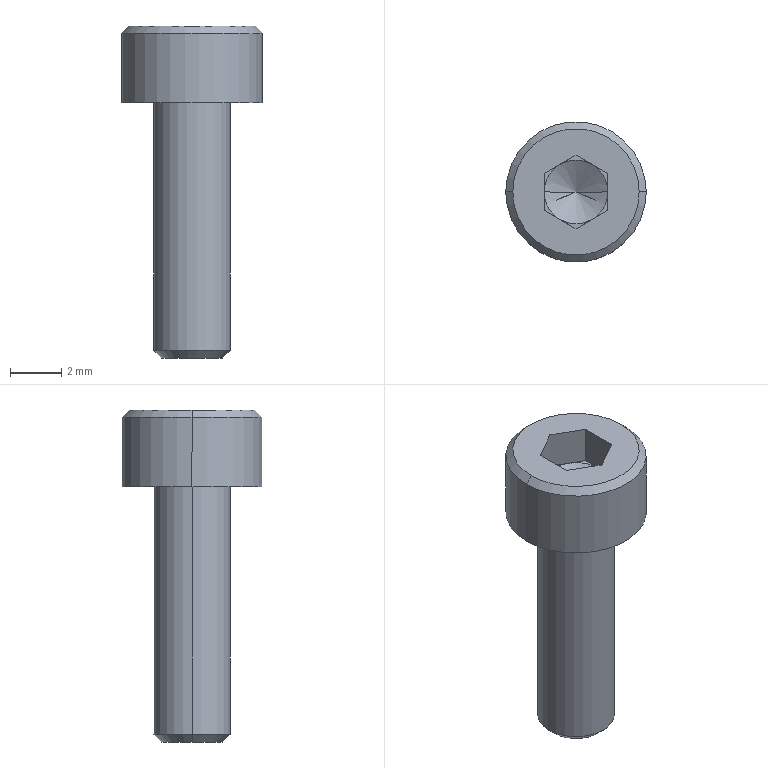Part | NX | features BREP 1 | 1 solid | 25 faces | box 5.5 x 5.5 x 13 mm | volume 131.617 mm3 | plane 15 | cone 6 | cylinder 4 | commonest cylinder face diameters 3 x2 5.5 x2
STEP:
#1=CARTESIAN_POINT('',(0.,0.,0.7783));
#2=VERTEX_POINT('',#1);
#3=CARTESIAN_POINT('',(1.25,0.,1.5));
#4=VERTEX_POINT('',#3);
#5=CARTESIAN_POINT('',(0.,0.,0.7783));
#6=DIRECTION('',(0.866,0.,0.5));
#7=VECTOR('',#6,1000.);
#8=LINE('',#5,#7);
#9=EDGE_CURVE('',#2,#4,#8,.T.);
#10=ORIENTED_EDGE('',*,*,#9,.F.);
#11=CARTESIAN_POINT('',(-1.25,0.,1.5));
#12=VERTEX_POINT('',#11);
#13=CARTESIAN_POINT('',(0.,0.,0.7783));
#14=DIRECTION('',(-0.866,0.,0.5));
#15=VECTOR('',#14,1000.);
#16=LINE('',#13,#15);
#17=EDGE_CURVE('',#2,#12,#16,.T.);
#18=ORIENTED_EDGE('',*,*,#17,.T.);
#19=CARTESIAN_POINT('',(-0.625,-1.083,1.5));
#20=VERTEX_POINT('',#19);
#21=CARTESIAN_POINT('',(0.,0.,1.5));
#22=DIRECTION('',(0.,0.,1.));
#23=DIRECTION('',(1.,0.,0.));
#24=AXIS2_PLACEMENT_3D('',#21,#22,#23);
#25=CIRCLE('',#24,1.25);
#26=EDGE_CURVE('',#12,#20,#25,.T.);
#27=ORIENTED_EDGE('',*,*,#26,.T.);
#28=CARTESIAN_POINT('',(0.625,-1.083,1.5));
#29=VERTEX_POINT('',#28);
#30=CARTESIAN_POINT('',(0.,0.,1.5));
#31=DIRECTION('',(0.,0.,1.));
#32=DIRECTION('',(1.,0.,0.));
#33=AXIS2_PLACEMENT_3D('',#30,#31,#32);
#34=CIRCLE('',#33,1.25);
#35=EDGE_CURVE('',#20,#29,#34,.T.);
#36=ORIENTED_EDGE('',*,*,#35,.T.);
#37=CARTESIAN_POINT('',(0.,0.,1.5));
#38=DIRECTION('',(0.,0.,1.));
#39=DIRECTION('',(1.,0.,0.));
#40=AXIS2_PLACEMENT_3D('',#37,#38,#39);
#41=CIRCLE('',#40,1.25);
#42=EDGE_CURVE('',#29,#4,#41,.T.);
#43=ORIENTED_EDGE('',*,*,#42,.T.);
#44=EDGE_LOOP('',(#10,#18,#27,#36,#43));
#45=FACE_BOUND('',#44,.T.);
#46=CARTESIAN_POINT('',(0.,0.,1000.778));
#47=DIRECTION('',(0.,0.,1.));
#48=DIRECTION('',(-1.,0.,0.));
#49=AXIS2_PLACEMENT_3D('',#46,#47,#48);
#50=CONICAL_SURFACE('',#49,1732.051,1.047);
#51=ADVANCED_FACE('',(#45),#50,.F.);
#52=CARTESIAN_POINT('',(2.75,0.,0.));
#53=VERTEX_POINT('',#52);
#54=CARTESIAN_POINT('',(-2.75,0.,0.));
#55=VERTEX_POINT('',#54);
#56=CARTESIAN_POINT('',(0.,0.,0.));
#57=DIRECTION('',(0.,0.,1.));
#58=DIRECTION('',(1.,0.,0.));
#59=AXIS2_PLACEMENT_3D('',#56,#57,#58);
#60=CIRCLE('',#59,2.75);
#61=EDGE_CURVE('',#53,#55,#60,.T.);
#62=ORIENTED_EDGE('',*,*,#61,.T.);
#63=CARTESIAN_POINT('',(-2.75,0.,2.725));
#64=VERTEX_POINT('',#63);
#65=CARTESIAN_POINT('',(-2.75,0.,0.));
#66=DIRECTION('',(0.,0.,1.));
#67=VECTOR('',#66,1000.);
#68=LINE('',#65,#67);
#69=EDGE_CURVE('',#55,#64,#68,.T.);
#70=ORIENTED_EDGE('',*,*,#69,.T.);
#71=CARTESIAN_POINT('',(2.75,0.,2.725));
#72=VERTEX_POINT('',#71);
#73=CARTESIAN_POINT('',(0.,0.,2.725));
#74=DIRECTION('',(0.,0.,1.));
#75=DIRECTION('',(1.,0.,0.));
#76=AXIS2_PLACEMENT_3D('',#73,#74,#75);
#77=CIRCLE('',#76,2.75);
#78=EDGE_CURVE('',#72,#64,#77,.T.);
#79=ORIENTED_EDGE('',*,*,#78,.F.);
#80=CARTESIAN_POINT('',(2.75,0.,0.));
#81=DIRECTION('',(0.,0.,1.));
#82=VECTOR('',#81,1000.);
#83=LINE('',#80,#82);
#84=EDGE_CURVE('',#53,#72,#83,.T.);
#85=ORIENTED_EDGE('',*,*,#84,.F.);
#86=EDGE_LOOP('',(#62,#70,#79,#85));
#87=FACE_BOUND('',#86,.T.);
#88=CARTESIAN_POINT('',(0.,0.,0.));
#89=DIRECTION('',(0.,0.,1.));
#90=DIRECTION('',(-1.,0.,0.));
#91=AXIS2_PLACEMENT_3D('',#88,#89,#90);
#92=CYLINDRICAL_SURFACE('',#91,2.75);
#93=ADVANCED_FACE('',(#87),#92,.T.);
#94=CARTESIAN_POINT('',(2.475,0.,3.));
#95=VERTEX_POINT('',#94);
#96=CARTESIAN_POINT('',(-2.475,0.,3.));
#97=VERTEX_POINT('',#96);
#98=CARTESIAN_POINT('',(0.,0.,3.));
#99=DIRECTION('',(0.,0.,1.));
#100=DIRECTION('',(1.,0.,0.));
#101=AXIS2_PLACEMENT_3D('',#98,#99,#100);
#102=CIRCLE('',#101,2.475);
#103=EDGE_CURVE('',#95,#97,#102,.T.);
#104=ORIENTED_EDGE('',*,*,#103,.F.);
#105=CARTESIAN_POINT('',(2.75,0.,2.725));
#106=DIRECTION('',(0.7071,0.,-0.7071));
#107=VECTOR('',#106,1000.);
#108=LINE('',#105,#107);
#109=EDGE_CURVE('',#72,#95,#108,.F.);
#110=ORIENTED_EDGE('',*,*,#109,.F.);
#111=ORIENTED_EDGE('',*,*,#78,.T.);
#112=CARTESIAN_POINT('',(-2.75,0.,2.725));
#113=DIRECTION('',(-0.7071,0.,-0.7071));
#114=VECTOR('',#113,1000.);
#115=LINE('',#112,#114);
#116=EDGE_CURVE('',#64,#97,#115,.F.);
#117=ORIENTED_EDGE('',*,*,#116,.T.);
#118=EDGE_LOOP('',(#104,#110,#111,#117));
#119=FACE_BOUND('',#118,.T.);
#120=CARTESIAN_POINT('',(0.,0.,2.725));
#121=DIRECTION('',(0.,0.,-1.));
#122=DIRECTION('',(1.,0.,0.));
#123=AXIS2_PLACEMENT_3D('',#120,#121,#122);
#124=CONICAL_SURFACE('',#123,2.75,0.7854);
#125=ADVANCED_FACE('',(#119),#124,.T.);
#126=CARTESIAN_POINT('',(1.194,0.,-10.));
#127=VERTEX_POINT('',#126);
#128=CARTESIAN_POINT('',(-1.194,0.,-10.));
#129=VERTEX_POINT('',#128);
#130=CARTESIAN_POINT('',(0.,0.,-10.));
#131=DIRECTION('',(0.,0.,1.));
#132=DIRECTION('',(1.,0.,0.));
#133=AXIS2_PLACEMENT_3D('',#130,#131,#132);
#134=CIRCLE('',#133,1.194);
#135=EDGE_CURVE('',#127,#129,#134,.T.);
#136=ORIENTED_EDGE('',*,*,#135,.T.);
#137=CARTESIAN_POINT('',(-1.5,0.,-9.694));
#138=VERTEX_POINT('',#137);
#139=CARTESIAN_POINT('',(-1.194,0.,-10.));
#140=DIRECTION('',(-0.7071,0.,0.7071));
#141=VECTOR('',#140,1000.);
#142=LINE('',#139,#141);
#143=EDGE_CURVE('',#129,#138,#142,.T.);
#144=ORIENTED_EDGE('',*,*,#143,.T.);
#145=CARTESIAN_POINT('',(1.5,0.,-9.694));
#146=VERTEX_POINT('',#145);
#147=CARTESIAN_POINT('',(0.,0.,-9.694));
#148=DIRECTION('',(0.,0.,1.));
#149=DIRECTION('',(1.,0.,0.));
#150=AXIS2_PLACEMENT_3D('',#147,#148,#149);
#151=CIRCLE('',#150,1.5);
#152=EDGE_CURVE('',#146,#138,#151,.T.);
#153=ORIENTED_EDGE('',*,*,#152,.F.);
#154=CARTESIAN_POINT('',(1.194,0.,-10.));
#155=DIRECTION('',(0.7071,0.,0.7071));
#156=VECTOR('',#155,1000.);
#157=LINE('',#154,#156);
#158=EDGE_CURVE('',#127,#146,#157,.T.);
#159=ORIENTED_EDGE('',*,*,#158,.F.);
#160=EDGE_LOOP('',(#136,#144,#153,#159));
#161=FACE_BOUND('',#160,.T.);
#162=CARTESIAN_POINT('',(0.,0.,-10.));
#163=DIRECTION('',(0.,0.,1.));
#164=DIRECTION('',(-1.,0.,0.));
#165=AXIS2_PLACEMENT_3D('',#162,#163,#164);
#166=CONICAL_SURFACE('',#165,1.194,0.7854);
#167=ADVANCED_FACE('',(#161),#166,.T.);
#168=ORIENTED_EDGE('',*,*,#152,.T.);
#169=CARTESIAN_POINT('',(-1.5,0.,0.));
#170=VERTEX_POINT('',#169);
#171=CARTESIAN_POINT('',(-1.5,0.,-10.));
#172=DIRECTION('',(0.,0.,1.));
#173=VECTOR('',#172,1000.);
#174=LINE('',#171,#173);
#175=EDGE_CURVE('',#138,#170,#174,.T.);
#176=ORIENTED_EDGE('',*,*,#175,.T.);
#177=CARTESIAN_POINT('',(1.5,0.,0.));
#178=VERTEX_POINT('',#177);
#179=CARTESIAN_POINT('',(0.,0.,0.));
#180=DIRECTION('',(0.,0.,1.));
#181=DIRECTION('',(1.,0.,0.));
#182=AXIS2_PLACEMENT_3D('',#179,#180,#181);
#183=CIRCLE('',#182,1.5);
#184=EDGE_CURVE('',#178,#170,#183,.T.);
#185=ORIENTED_EDGE('',*,*,#184,.F.);
#186=CARTESIAN_POINT('',(1.5,0.,-10.));
#187=DIRECTION('',(0.,0.,1.));
#188=VECTOR('',#187,1000.);
#189=LINE('',#186,#188);
#190=EDGE_CURVE('',#146,#178,#189,.T.);
#191=ORIENTED_EDGE('',*,*,#190,.F.);
#192=EDGE_LOOP('',(#168,#176,#185,#191));
#193=FACE_BOUND('',#192,.T.);
#194=CARTESIAN_POINT('',(0.,0.,-10.));
#195=DIRECTION('',(0.,0.,1.));
#196=DIRECTION('',(-1.,0.,0.));
#197=AXIS2_PLACEMENT_3D('',#194,#195,#196);
#198=CYLINDRICAL_SURFACE('',#197,1.5);
#199=ADVANCED_FACE('',(#193),#198,.T.);
#200=CARTESIAN_POINT('',(0.625,1.083,1.5));
#201=VERTEX_POINT('',#200);
#202=CARTESIAN_POINT('',(0.,0.,1.5));
#203=DIRECTION('',(0.,0.,1.));
#204=DIRECTION('',(1.,0.,0.));
#205=AXIS2_PLACEMENT_3D('',#202,#203,#204);
#206=CIRCLE('',#205,1.25);
#207=EDGE_CURVE('',#4,#201,#206,.T.);
#208=ORIENTED_EDGE('',*,*,#207,.F.);
#209=CARTESIAN_POINT('',(1.25,0.7217,1.5));
#210=VERTEX_POINT('',#209);
#211=CARTESIAN_POINT('',(1.25,-0.7217,1.5));
#212=DIRECTION('',(0.,1.,0.));
#213=VECTOR('',#212,1000.);
#214=LINE('',#211,#213);
#215=EDGE_CURVE('',#4,#210,#214,.T.);
#216=ORIENTED_EDGE('',*,*,#215,.T.);
#217=CARTESIAN_POINT('',(1.25,0.7217,1.5));
#218=DIRECTION('',(-0.866,0.5,0.));
#219=VECTOR('',#218,1000.);
#220=LINE('',#217,#219);
#221=EDGE_CURVE('',#210,#201,#220,.T.);
#222=ORIENTED_EDGE('',*,*,#221,.T.);
#223=EDGE_LOOP('',(#208,#216,#222));
#224=FACE_BOUND('',#223,.T.);
#225=CARTESIAN_POINT('',(0.,0.,1.5));
#226=DIRECTION('',(0.,0.,1.));
#227=DIRECTION('',(-1.,0.,0.));
#228=AXIS2_PLACEMENT_3D('',#225,#226,#227);
#229=PLANE('',#228);
#230=ADVANCED_FACE('',(#224),#229,.T.);
#231=CARTESIAN_POINT('',(-0.625,1.083,1.5));
#232=VERTEX_POINT('',#231);
#233=CARTESIAN_POINT('',(0.,0.,1.5));
#234=DIRECTION('',(0.,0.,1.));
#235=DIRECTION('',(1.,0.,0.));
#236=AXIS2_PLACEMENT_3D('',#233,#234,#235);
#237=CIRCLE('',#236,1.25);
#238=EDGE_CURVE('',#201,#232,#237,.T.);
#239=ORIENTED_EDGE('',*,*,#238,.F.);
#240=CARTESIAN_POINT('',(0.,1.443,1.5));
#241=VERTEX_POINT('',#240);
#242=CARTESIAN_POINT('',(1.25,0.7217,1.5));
#243=DIRECTION('',(-0.866,0.5,0.));
#244=VECTOR('',#243,1000.);
#245=LINE('',#242,#244);
#246=EDGE_CURVE('',#201,#241,#245,.T.);
#247=ORIENTED_EDGE('',*,*,#246,.T.);
#248=CARTESIAN_POINT('',(0.,1.443,1.5));
#249=DIRECTION('',(-0.866,-0.5,0.));
#250=VECTOR('',#249,1000.);
#251=LINE('',#248,#250);
#252=EDGE_CURVE('',#241,#232,#251,.T.);
#253=ORIENTED_EDGE('',*,*,#252,.T.);
#254=EDGE_LOOP('',(#239,#247,#253));
#255=FACE_BOUND('',#254,.T.);
#256=CARTESIAN_POINT('',(0.,0.,1.5));
#257=DIRECTION('',(0.,0.,1.));
#258=DIRECTION('',(-1.,0.,0.));
#259=AXIS2_PLACEMENT_3D('',#256,#257,#258);
#260=PLANE('',#259);
#261=ADVANCED_FACE('',(#255),#260,.T.);
#262=CARTESIAN_POINT('',(0.,0.,1.5));
#263=DIRECTION('',(0.,0.,1.));
#264=DIRECTION('',(1.,0.,0.));
#265=AXIS2_PLACEMENT_3D('',#262,#263,#264);
#266=CIRCLE('',#265,1.25);
#267=EDGE_CURVE('',#232,#12,#266,.T.);
#268=ORIENTED_EDGE('',*,*,#267,.F.);
#269=CARTESIAN_POINT('',(-1.25,0.7217,1.5));
#270=VERTEX_POINT('',#269);
#271=CARTESIAN_POINT('',(0.,1.443,1.5));
#272=DIRECTION('',(-0.866,-0.5,0.));
#273=VECTOR('',#272,1000.);
#274=LINE('',#271,#273);
#275=EDGE_CURVE('',#232,#270,#274,.T.);
#276=ORIENTED_EDGE('',*,*,#275,.T.);
#277=CARTESIAN_POINT('',(-1.25,0.7217,1.5));
#278=DIRECTION('',(0.,-1.,0.));
#279=VECTOR('',#278,1000.);
#280=LINE('',#277,#279);
#281=EDGE_CURVE('',#270,#12,#280,.T.);
#282=ORIENTED_EDGE('',*,*,#281,.T.);
#283=EDGE_LOOP('',(#268,#276,#282));
#284=FACE_BOUND('',#283,.T.);
#285=CARTESIAN_POINT('',(0.,0.,1.5));
#286=DIRECTION('',(0.,0.,1.));
#287=DIRECTION('',(-1.,0.,0.));
#288=AXIS2_PLACEMENT_3D('',#285,#286,#287);
#289=PLANE('',#288);
#290=ADVANCED_FACE('',(#284),#289,.T.);
#291=ORIENTED_EDGE('',*,*,#26,.F.);
#292=CARTESIAN_POINT('',(-1.25,-0.7217,1.5));
#293=VERTEX_POINT('',#292);
#294=CARTESIAN_POINT('',(-1.25,0.7217,1.5));
#295=DIRECTION('',(0.,-1.,0.));
#296=VECTOR('',#295,1000.);
#297=LINE('',#294,#296);
#298=EDGE_CURVE('',#12,#293,#297,.T.);
#299=ORIENTED_EDGE('',*,*,#298,.T.);
#300=CARTESIAN_POINT('',(-1.25,-0.7217,1.5));
#301=DIRECTION('',(0.866,-0.5,0.));
#302=VECTOR('',#301,1000.);
#303=LINE('',#300,#302);
#304=EDGE_CURVE('',#293,#20,#303,.T.);
#305=ORIENTED_EDGE('',*,*,#304,.T.);
#306=EDGE_LOOP('',(#291,#299,#305));
#307=FACE_BOUND('',#306,.T.);
#308=CARTESIAN_POINT('',(0.,0.,1.5));
#309=DIRECTION('',(0.,0.,1.));
#310=DIRECTION('',(-1.,0.,0.));
#311=AXIS2_PLACEMENT_3D('',#308,#309,#310);
#312=PLANE('',#311);
#313=ADVANCED_FACE('',(#307),#312,.T.);
#314=ORIENTED_EDGE('',*,*,#35,.F.);
#315=CARTESIAN_POINT('',(0.,-1.443,1.5));
#316=VERTEX_POINT('',#315);
#317=CARTESIAN_POINT('',(-1.25,-0.7217,1.5));
#318=DIRECTION('',(0.866,-0.5,0.));
#319=VECTOR('',#318,1000.);
#320=LINE('',#317,#319);
#321=EDGE_CURVE('',#20,#316,#320,.T.);
#322=ORIENTED_EDGE('',*,*,#321,.T.);
#323=CARTESIAN_POINT('',(0.,-1.443,1.5));
#324=DIRECTION('',(0.866,0.5,0.));
#325=VECTOR('',#324,1000.);
#326=LINE('',#323,#325);
#327=EDGE_CURVE('',#316,#29,#326,.T.);
#328=ORIENTED_EDGE('',*,*,#327,.T.);
#329=EDGE_LOOP('',(#314,#322,#328));
#330=FACE_BOUND('',#329,.T.);
#331=CARTESIAN_POINT('',(0.,0.,1.5));
#332=DIRECTION('',(0.,0.,1.));
#333=DIRECTION('',(-1.,0.,0.));
#334=AXIS2_PLACEMENT_3D('',#331,#332,#333);
#335=PLANE('',#334);
#336=ADVANCED_FACE('',(#330),#335,.T.);
#337=ORIENTED_EDGE('',*,*,#175,.F.);
#338=CARTESIAN_POINT('',(0.,0.,-9.694));
#339=DIRECTION('',(0.,0.,1.));
#340=DIRECTION('',(1.,0.,0.));
#341=AXIS2_PLACEMENT_3D('',#338,#339,#340);
#342=CIRCLE('',#341,1.5);
#343=EDGE_CURVE('',#138,#146,#342,.T.);
#344=ORIENTED_EDGE('',*,*,#343,.T.);
#345=ORIENTED_EDGE('',*,*,#190,.T.);
#346=CARTESIAN_POINT('',(0.,0.,0.));
#347=DIRECTION('',(0.,0.,1.));
#348=DIRECTION('',(1.,0.,0.));
#349=AXIS2_PLACEMENT_3D('',#346,#347,#348);
#350=CIRCLE('',#349,1.5);
#351=EDGE_CURVE('',#170,#178,#350,.T.);
#352=ORIENTED_EDGE('',*,*,#351,.F.);
#353=EDGE_LOOP('',(#337,#344,#345,#352));
#354=FACE_BOUND('',#353,.T.);
#355=CARTESIAN_POINT('',(0.,0.,-10.));
#356=DIRECTION('',(0.,0.,1.));
#357=DIRECTION('',(-1.,0.,0.));
#358=AXIS2_PLACEMENT_3D('',#355,#356,#357);
#359=CYLINDRICAL_SURFACE('',#358,1.5);
#360=ADVANCED_FACE('',(#354),#359,.T.);
#361=ORIENTED_EDGE('',*,*,#143,.F.);
#362=CARTESIAN_POINT('',(0.,0.,-10.));
#363=DIRECTION('',(0.,0.,1.));
#364=DIRECTION('',(1.,0.,0.));
#365=AXIS2_PLACEMENT_3D('',#362,#363,#364);
#366=CIRCLE('',#365,1.194);
#367=EDGE_CURVE('',#129,#127,#366,.T.);
#368=ORIENTED_EDGE('',*,*,#367,.T.);
#369=ORIENTED_EDGE('',*,*,#158,.T.);
#370=ORIENTED_EDGE('',*,*,#343,.F.);
#371=EDGE_LOOP('',(#361,#368,#369,#370));
#372=FACE_BOUND('',#371,.T.);
#373=CARTESIAN_POINT('',(0.,0.,-10.));
#374=DIRECTION('',(0.,0.,1.));
#375=DIRECTION('',(-1.,0.,0.));
#376=AXIS2_PLACEMENT_3D('',#373,#374,#375);
#377=CONICAL_SURFACE('',#376,1.194,0.7854);
#378=ADVANCED_FACE('',(#372),#377,.T.);
#379=ORIENTED_EDGE('',*,*,#135,.F.);
#380=ORIENTED_EDGE('',*,*,#367,.F.);
#381=EDGE_LOOP('',(#379,#380));
#382=FACE_BOUND('',#381,.T.);
#383=CARTESIAN_POINT('',(0.,1.194,-10.));
#384=DIRECTION('',(0.,0.,1.));
#385=DIRECTION('',(-1.,0.,0.));
#386=AXIS2_PLACEMENT_3D('',#383,#384,#385);
#387=PLANE('',#386);
#388=ADVANCED_FACE('',(#382),#387,.F.);
#389=CARTESIAN_POINT('',(0.,-1.443,3.));
#390=VERTEX_POINT('',#389);
#391=CARTESIAN_POINT('',(1.25,-0.7217,3.));
#392=VERTEX_POINT('',#391);
#393=CARTESIAN_POINT('',(0.,-1.443,3.));
#394=DIRECTION('',(0.866,0.5,0.));
#395=VECTOR('',#394,1000.);
#396=LINE('',#393,#395);
#397=EDGE_CURVE('',#390,#392,#396,.T.);
#398=ORIENTED_EDGE('',*,*,#397,.F.);
#399=CARTESIAN_POINT('',(-1.25,-0.7217,3.));
#400=VERTEX_POINT('',#399);
#401=CARTESIAN_POINT('',(-1.25,-0.7217,3.));
#402=DIRECTION('',(0.866,-0.5,0.));
#403=VECTOR('',#402,1000.);
#404=LINE('',#401,#403);
#405=EDGE_CURVE('',#400,#390,#404,.T.);
#406=ORIENTED_EDGE('',*,*,#405,.F.);
#407=CARTESIAN_POINT('',(-1.25,0.7217,3.));
#408=VERTEX_POINT('',#407);
#409=CARTESIAN_POINT('',(-1.25,0.7217,3.));
#410=DIRECTION('',(0.,-1.,0.));
#411=VECTOR('',#410,1000.);
#412=LINE('',#409,#411);
#413=EDGE_CURVE('',#408,#400,#412,.T.);
#414=ORIENTED_EDGE('',*,*,#413,.F.);
#415=CARTESIAN_POINT('',(0.,1.443,3.));
#416=VERTEX_POINT('',#415);
#417=CARTESIAN_POINT('',(0.,1.443,3.));
#418=DIRECTION('',(-0.866,-0.5,0.));
#419=VECTOR('',#418,1000.);
#420=LINE('',#417,#419);
#421=EDGE_CURVE('',#416,#408,#420,.T.);
#422=ORIENTED_EDGE('',*,*,#421,.F.);
#423=CARTESIAN_POINT('',(1.25,0.7217,3.));
#424=VERTEX_POINT('',#423);
#425=CARTESIAN_POINT('',(1.25,0.7217,3.));
#426=DIRECTION('',(-0.866,0.5,0.));
#427=VECTOR('',#426,1000.);
#428=LINE('',#425,#427);
#429=EDGE_CURVE('',#424,#416,#428,.T.);
#430=ORIENTED_EDGE('',*,*,#429,.F.);
#431=CARTESIAN_POINT('',(1.25,-0.7217,3.));
#432=DIRECTION('',(0.,1.,0.));
#433=VECTOR('',#432,1000.);
#434=LINE('',#431,#433);
#435=EDGE_CURVE('',#392,#424,#434,.T.);
#436=ORIENTED_EDGE('',*,*,#435,.F.);
#437=EDGE_LOOP('',(#398,#406,#414,#422,#430,#436));
#438=FACE_BOUND('',#437,.T.);
#439=CARTESIAN_POINT('',(0.,0.,3.));
#440=DIRECTION('',(0.,0.,1.));
#441=DIRECTION('',(1.,0.,0.));
#442=AXIS2_PLACEMENT_3D('',#439,#440,#441);
#443=CIRCLE('',#442,2.475);
#444=EDGE_CURVE('',#97,#95,#443,.T.);
#445=ORIENTED_EDGE('',*,*,#444,.T.);
#446=ORIENTED_EDGE('',*,*,#103,.T.);
#447=EDGE_LOOP('',(#445,#446));
#448=FACE_BOUND('',#447,.T.);
#449=CARTESIAN_POINT('',(0.,0.,3.));
#450=DIRECTION('',(0.,0.,-1.));
#451=DIRECTION('',(1.,0.,0.));
#452=AXIS2_PLACEMENT_3D('',#449,#450,#451);
#453=PLANE('',#452);
#454=ADVANCED_FACE('',(#438,#448),#453,.F.);
#455=ORIENTED_EDGE('',*,*,#109,.T.);
#456=ORIENTED_EDGE('',*,*,#444,.F.);
#457=ORIENTED_EDGE('',*,*,#116,.F.);
#458=CARTESIAN_POINT('',(0.,0.,2.725));
#459=DIRECTION('',(0.,0.,1.));
#460=DIRECTION('',(1.,0.,0.));
#461=AXIS2_PLACEMENT_3D('',#458,#459,#460);
#462=CIRCLE('',#461,2.75);
#463=EDGE_CURVE('',#64,#72,#462,.T.);
#464=ORIENTED_EDGE('',*,*,#463,.T.);
#465=EDGE_LOOP('',(#455,#456,#457,#464));
#466=FACE_BOUND('',#465,.T.);
#467=CARTESIAN_POINT('',(0.,0.,2.725));
#468=DIRECTION('',(0.,0.,-1.));
#469=DIRECTION('',(1.,0.,0.));
#470=AXIS2_PLACEMENT_3D('',#467,#468,#469);
#471=CONICAL_SURFACE('',#470,2.75,0.7854);
#472=ADVANCED_FACE('',(#466),#471,.T.);
#473=ORIENTED_EDGE('',*,*,#69,.F.);
#474=CARTESIAN_POINT('',(0.,0.,0.));
#475=DIRECTION('',(0.,0.,1.));
#476=DIRECTION('',(1.,0.,0.));
#477=AXIS2_PLACEMENT_3D('',#474,#475,#476);
#478=CIRCLE('',#477,2.75);
#479=EDGE_CURVE('',#55,#53,#478,.T.);
#480=ORIENTED_EDGE('',*,*,#479,.T.);
#481=ORIENTED_EDGE('',*,*,#84,.T.);
#482=ORIENTED_EDGE('',*,*,#463,.F.);
#483=EDGE_LOOP('',(#473,#480,#481,#482));
#484=FACE_BOUND('',#483,.T.);
#485=CARTESIAN_POINT('',(0.,0.,0.));
#486=DIRECTION('',(0.,0.,1.));
#487=DIRECTION('',(-1.,0.,0.));
#488=AXIS2_PLACEMENT_3D('',#485,#486,#487);
#489=CYLINDRICAL_SURFACE('',#488,2.75);
#490=ADVANCED_FACE('',(#484),#489,.T.);
#491=ORIENTED_EDGE('',*,*,#184,.T.);
#492=ORIENTED_EDGE('',*,*,#351,.T.);
#493=EDGE_LOOP('',(#491,#492));
#494=FACE_BOUND('',#493,.T.);
#495=ORIENTED_EDGE('',*,*,#61,.F.);
#496=ORIENTED_EDGE('',*,*,#479,.F.);
#497=EDGE_LOOP('',(#495,#496));
#498=FACE_BOUND('',#497,.T.);
#499=CARTESIAN_POINT('',(0.,2.75,0.));
#500=DIRECTION('',(0.,0.,1.));
#501=DIRECTION('',(-1.,0.,0.));
#502=AXIS2_PLACEMENT_3D('',#499,#500,#501);
#503=PLANE('',#502);
#504=ADVANCED_FACE('',(#494,#498),#503,.F.);
#505=ORIENTED_EDGE('',*,*,#405,.T.);
#506=CARTESIAN_POINT('',(0.,-1.443,1.5));
#507=DIRECTION('',(0.,0.,1.));
#508=VECTOR('',#507,1000.);
#509=LINE('',#506,#508);
#510=EDGE_CURVE('',#316,#390,#509,.T.);
#511=ORIENTED_EDGE('',*,*,#510,.F.);
#512=ORIENTED_EDGE('',*,*,#321,.F.);
#513=ORIENTED_EDGE('',*,*,#304,.F.);
#514=CARTESIAN_POINT('',(-1.25,-0.7217,1.5));
#515=DIRECTION('',(0.,0.,1.));
#516=VECTOR('',#515,1000.);
#517=LINE('',#514,#516);
#518=EDGE_CURVE('',#293,#400,#517,.T.);
#519=ORIENTED_EDGE('',*,*,#518,.T.);
#520=EDGE_LOOP('',(#505,#511,#512,#513,#519));
#521=FACE_BOUND('',#520,.T.);
#522=CARTESIAN_POINT('',(-1.25,-0.7217,1.5));
#523=DIRECTION('',(-0.5,-0.866,0.));
#524=DIRECTION('',(-0.866,0.5,0.));
#525=AXIS2_PLACEMENT_3D('',#522,#523,#524);
#526=PLANE('',#525);
#527=ADVANCED_FACE('',(#521),#526,.F.);
#528=ORIENTED_EDGE('',*,*,#413,.T.);
#529=ORIENTED_EDGE('',*,*,#518,.F.);
#530=ORIENTED_EDGE('',*,*,#298,.F.);
#531=ORIENTED_EDGE('',*,*,#281,.F.);
#532=CARTESIAN_POINT('',(-1.25,0.7217,1.5));
#533=DIRECTION('',(0.,0.,1.));
#534=VECTOR('',#533,1000.);
#535=LINE('',#532,#534);
#536=EDGE_CURVE('',#270,#408,#535,.T.);
#537=ORIENTED_EDGE('',*,*,#536,.T.);
#538=EDGE_LOOP('',(#528,#529,#530,#531,#537));
#539=FACE_BOUND('',#538,.T.);
#540=CARTESIAN_POINT('',(-1.25,0.7217,1.5));
#541=DIRECTION('',(-1.,0.,0.));
#542=DIRECTION('',(0.,0.,-1.));
#543=AXIS2_PLACEMENT_3D('',#540,#541,#542);
#544=PLANE('',#543);
#545=ADVANCED_FACE('',(#539),#544,.F.);
#546=ORIENTED_EDGE('',*,*,#421,.T.);
#547=ORIENTED_EDGE('',*,*,#536,.F.);
#548=ORIENTED_EDGE('',*,*,#275,.F.);
#549=ORIENTED_EDGE('',*,*,#252,.F.);
#550=CARTESIAN_POINT('',(0.,1.443,1.5));
#551=DIRECTION('',(0.,0.,1.));
#552=VECTOR('',#551,1000.);
#553=LINE('',#550,#552);
#554=EDGE_CURVE('',#241,#416,#553,.T.);
#555=ORIENTED_EDGE('',*,*,#554,.T.);
#556=EDGE_LOOP('',(#546,#547,#548,#549,#555));
#557=FACE_BOUND('',#556,.T.);
#558=CARTESIAN_POINT('',(0.,1.443,1.5));
#559=DIRECTION('',(-0.5,0.866,0.));
#560=DIRECTION('',(0.866,0.5,0.));
#561=AXIS2_PLACEMENT_3D('',#558,#559,#560);
#562=PLANE('',#561);
#563=ADVANCED_FACE('',(#557),#562,.F.);
#564=ORIENTED_EDGE('',*,*,#429,.T.);
#565=ORIENTED_EDGE('',*,*,#554,.F.);
#566=ORIENTED_EDGE('',*,*,#246,.F.);
#567=ORIENTED_EDGE('',*,*,#221,.F.);
#568=CARTESIAN_POINT('',(1.25,0.7217,1.5));
#569=DIRECTION('',(0.,0.,1.));
#570=VECTOR('',#569,1000.);
#571=LINE('',#568,#570);
#572=EDGE_CURVE('',#210,#424,#571,.T.);
#573=ORIENTED_EDGE('',*,*,#572,.T.);
#574=EDGE_LOOP('',(#564,#565,#566,#567,#573));
#575=FACE_BOUND('',#574,.T.);
#576=CARTESIAN_POINT('',(1.25,0.7217,1.5));
#577=DIRECTION('',(0.5,0.866,0.));
#578=DIRECTION('',(0.866,-0.5,0.));
#579=AXIS2_PLACEMENT_3D('',#576,#577,#578);
#580=PLANE('',#579);
#581=ADVANCED_FACE('',(#575),#580,.F.);
#582=ORIENTED_EDGE('',*,*,#435,.T.);
#583=ORIENTED_EDGE('',*,*,#572,.F.);
#584=ORIENTED_EDGE('',*,*,#215,.F.);
#585=CARTESIAN_POINT('',(1.25,-0.7217,1.5));
#586=VERTEX_POINT('',#585);
#587=CARTESIAN_POINT('',(1.25,-0.7217,1.5));
#588=DIRECTION('',(0.,1.,0.));
#589=VECTOR('',#588,1000.);
#590=LINE('',#587,#589);
#591=EDGE_CURVE('',#586,#4,#590,.T.);
#592=ORIENTED_EDGE('',*,*,#591,.F.);
#593=CARTESIAN_POINT('',(1.25,-0.7217,1.5));
#594=DIRECTION('',(0.,0.,1.));
#595=VECTOR('',#594,1000.);
#596=LINE('',#593,#595);
#597=EDGE_CURVE('',#586,#392,#596,.T.);
#598=ORIENTED_EDGE('',*,*,#597,.T.);
#599=EDGE_LOOP('',(#582,#583,#584,#592,#598));
#600=FACE_BOUND('',#599,.T.);
#601=CARTESIAN_POINT('',(1.25,-0.7217,1.5));
#602=DIRECTION('',(1.,0.,0.));
#603=DIRECTION('',(0.,0.,1.));
#604=AXIS2_PLACEMENT_3D('',#601,#602,#603);
#605=PLANE('',#604);
#606=ADVANCED_FACE('',(#600),#605,.F.);
#607=ORIENTED_EDGE('',*,*,#397,.T.);
#608=ORIENTED_EDGE('',*,*,#597,.F.);
#609=CARTESIAN_POINT('',(0.,-1.443,1.5));
#610=DIRECTION('',(0.866,0.5,0.));
#611=VECTOR('',#610,1000.);
#612=LINE('',#609,#611);
#613=EDGE_CURVE('',#29,#586,#612,.T.);
#614=ORIENTED_EDGE('',*,*,#613,.F.);
#615=ORIENTED_EDGE('',*,*,#327,.F.);
#616=ORIENTED_EDGE('',*,*,#510,.T.);
#617=EDGE_LOOP('',(#607,#608,#614,#615,#616));
#618=FACE_BOUND('',#617,.T.);
#619=CARTESIAN_POINT('',(0.,-1.443,1.5));
#620=DIRECTION('',(0.5,-0.866,0.));
#621=DIRECTION('',(-0.866,-0.5,0.));
#622=AXIS2_PLACEMENT_3D('',#619,#620,#621);
#623=PLANE('',#622);
#624=ADVANCED_FACE('',(#618),#623,.F.);
#625=ORIENTED_EDGE('',*,*,#42,.F.);
#626=ORIENTED_EDGE('',*,*,#613,.T.);
#627=ORIENTED_EDGE('',*,*,#591,.T.);
#628=EDGE_LOOP('',(#625,#626,#627));
#629=FACE_BOUND('',#628,.T.);
#630=CARTESIAN_POINT('',(0.,0.,1.5));
#631=DIRECTION('',(0.,0.,1.));
#632=DIRECTION('',(-1.,0.,0.));
#633=AXIS2_PLACEMENT_3D('',#630,#631,#632);
#634=PLANE('',#633);
#635=ADVANCED_FACE('',(#629),#634,.T.);
#636=ORIENTED_EDGE('',*,*,#17,.F.);
#637=ORIENTED_EDGE('',*,*,#9,.T.);
#638=ORIENTED_EDGE('',*,*,#207,.T.);
#639=ORIENTED_EDGE('',*,*,#238,.T.);
#640=ORIENTED_EDGE('',*,*,#267,.T.);
#641=EDGE_LOOP('',(#636,#637,#638,#639,#640));
#642=FACE_BOUND('',#641,.T.);
#643=CARTESIAN_POINT('',(0.,0.,1000.778));
#644=DIRECTION('',(0.,0.,1.));
#645=DIRECTION('',(-1.,0.,0.));
#646=AXIS2_PLACEMENT_3D('',#643,#644,#645);
#647=CONICAL_SURFACE('',#646,1732.051,1.047);
#648=ADVANCED_FACE('',(#642),#647,.F.);
#649=CLOSED_SHELL('',(#51,#93,#125,#167,#199,#230,#261,#290,#313,#336,#360,#378,#388,#454,#472,#490,#504,#527,#545,#563,#581,#606,#624,#635,#648));
#650=MANIFOLD_SOLID_BREP('',#649);
#651=(LENGTH_UNIT()NAMED_UNIT(*)SI_UNIT(.MILLI.,.METRE.));
#652=UNCERTAINTY_MEASURE_WITH_UNIT(LENGTH_MEASURE(0.00001),#651,'','');
#653=(NAMED_UNIT(*)PLANE_ANGLE_UNIT()SI_UNIT($,.RADIAN.));
#654=(NAMED_UNIT(*)SI_UNIT($,.STERADIAN.)SOLID_ANGLE_UNIT());
#655=(GEOMETRIC_REPRESENTATION_CONTEXT(3)GLOBAL_UNCERTAINTY_ASSIGNED_CONTEXT((#652))GLOBAL_UNIT_ASSIGNED_CONTEXT((#651,#653,#654))REPRESENTATION_CONTEXT('',''));
#656=ADVANCED_BREP_SHAPE_REPRESENTATION('',(#650),#655);